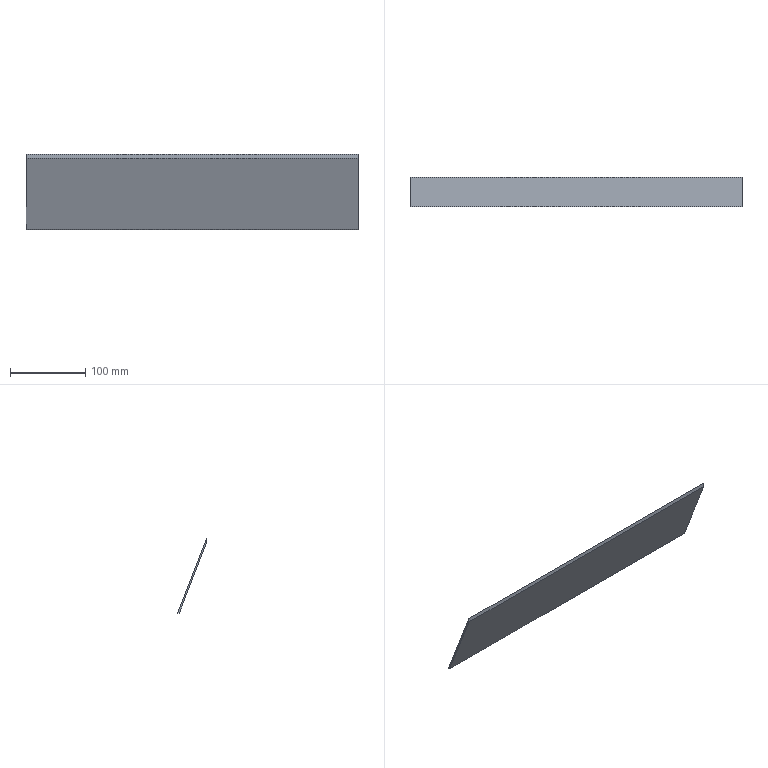Part | NX | features solid 2 | 1 solid | 6 faces | box 440 x 38.653 x 100.695 mm | volume 91707 mm3 | plane 5 | spline 1
STEP:
#1=CARTESIAN_POINT('',(-220.,-25.961,-130.224));
#2=VERTEX_POINT('',#1);
#3=CARTESIAN_POINT('',(-220.,-23.351,-131.441));
#4=VERTEX_POINT('',#3);
#5=CARTESIAN_POINT('',(-220.,730.,-482.734));
#6=DIRECTION('',(0.,-0.9063,0.4226));
#7=VECTOR('',#6,1000.);
#8=LINE('',#5,#7);
#9=EDGE_CURVE('',#2,#4,#8,.F.);
#10=ORIENTED_EDGE('',*,*,#9,.F.);
#11=CARTESIAN_POINT('',(-220.,-62.002,-36.334));
#12=VERTEX_POINT('',#11);
#13=CARTESIAN_POINT('',(-220.,-33.813,-109.769));
#14=DIRECTION('',(0.,-0.3584,0.9336));
#15=VECTOR('',#14,1000.);
#16=LINE('',#13,#15);
#17=EDGE_CURVE('',#2,#12,#16,.T.);
#18=ORIENTED_EDGE('',*,*,#17,.T.);
#19=CARTESIAN_POINT('',(-220.,-62.002,-30.753));
#20=VERTEX_POINT('',#19);
#21=CARTESIAN_POINT('',(-220.,-62.002,-33.544));
#22=DIRECTION('',(0.,0.,1.));
#23=VECTOR('',#22,1000.);
#24=LINE('',#21,#23);
#25=EDGE_CURVE('',#12,#20,#24,.T.);
#26=ORIENTED_EDGE('',*,*,#25,.T.);
#27=CARTESIAN_POINT('',(-220.,-31.946,-109.052));
#28=DIRECTION('',(0.,-0.3584,0.9336));
#29=VECTOR('',#28,1000.);
#30=LINE('',#27,#29);
#31=EDGE_CURVE('',#4,#20,#30,.T.);
#32=ORIENTED_EDGE('',*,*,#31,.F.);
#33=EDGE_LOOP('',(#10,#18,#26,#32));
#34=FACE_BOUND('',#33,.T.);
#35=CARTESIAN_POINT('',(-220.,-33.813,-109.769));
#36=DIRECTION('',(-1.,0.,0.));
#37=DIRECTION('',(0.,-0.3584,0.9336));
#38=AXIS2_PLACEMENT_3D('',#35,#36,#37);
#39=PLANE('',#38);
#40=ADVANCED_FACE('',(#34),#39,.T.);
#41=ORIENTED_EDGE('',*,*,#25,.F.);
#42=CARTESIAN_POINT('',(220.,-62.,-36.338));
#43=VERTEX_POINT('',#42);
#44=CARTESIAN_POINT('',(-220.,-62.002,-36.334));
#45=CARTESIAN_POINT('',(-73.333,-62.009,-36.315));
#46=CARTESIAN_POINT('',(73.333,-62.,-36.338));
#47=CARTESIAN_POINT('',(220.,-62.,-36.338));
#48=B_SPLINE_CURVE_WITH_KNOTS('',3,(#44,#45,#46,#47),.UNSPECIFIED.,.F.,.F.,(4,4),(0.,0.44),.UNSPECIFIED.);
#49=EDGE_CURVE('',#12,#43,#48,.T.);
#50=ORIENTED_EDGE('',*,*,#49,.T.);
#51=CARTESIAN_POINT('',(220.,-62.,-30.758));
#52=VERTEX_POINT('',#51);
#53=CARTESIAN_POINT('',(220.,-62.,-33.548));
#54=DIRECTION('',(0.,0.,1.));
#55=VECTOR('',#54,1000.);
#56=LINE('',#53,#55);
#57=EDGE_CURVE('',#43,#52,#56,.T.);
#58=ORIENTED_EDGE('',*,*,#57,.T.);
#59=CARTESIAN_POINT('',(-220.,-62.002,-30.753));
#60=CARTESIAN_POINT('',(-73.333,-62.009,-30.734));
#61=CARTESIAN_POINT('',(73.333,-62.,-30.758));
#62=CARTESIAN_POINT('',(220.,-62.,-30.758));
#63=B_SPLINE_CURVE_WITH_KNOTS('',3,(#59,#60,#61,#62),.UNSPECIFIED.,.F.,.F.,(4,4),(0.,0.44),.UNSPECIFIED.);
#64=EDGE_CURVE('',#20,#52,#63,.T.);
#65=ORIENTED_EDGE('',*,*,#64,.F.);
#66=EDGE_LOOP('',(#41,#50,#58,#65));
#67=FACE_BOUND('',#66,.T.);
#68=CARTESIAN_POINT('',(-220.,-62.002,-36.372));
#69=CARTESIAN_POINT('',(-220.,-62.002,-30.714));
#70=CARTESIAN_POINT('',(-73.333,-62.009,-36.372));
#71=CARTESIAN_POINT('',(-73.333,-62.009,-30.714));
#72=CARTESIAN_POINT('',(73.333,-62.,-36.372));
#73=CARTESIAN_POINT('',(73.333,-62.,-30.714));
#74=CARTESIAN_POINT('',(220.,-62.,-36.372));
#75=CARTESIAN_POINT('',(220.,-62.,-30.714));
#76=B_SPLINE_SURFACE_WITH_KNOTS('',3,1,((#68,#69),(#70,#71),(#72,#73),(#74,#75)),.SURF_OF_LINEAR_EXTRUSION.,.F.,.F.,.F.,(4,4),(2,2),(0.04348,1.957),(0.,1.),.PIECEWISE_BEZIER_KNOTS.);
#77=ADVANCED_FACE('',(#67),#76,.T.);
#78=ORIENTED_EDGE('',*,*,#57,.F.);
#79=CARTESIAN_POINT('',(220.,-25.961,-130.224));
#80=VERTEX_POINT('',#79);
#81=CARTESIAN_POINT('',(220.,-33.813,-109.769));
#82=DIRECTION('',(0.,-0.3584,0.9336));
#83=VECTOR('',#82,1000.);
#84=LINE('',#81,#83);
#85=EDGE_CURVE('',#80,#43,#84,.T.);
#86=ORIENTED_EDGE('',*,*,#85,.F.);
#87=CARTESIAN_POINT('',(220.,-23.351,-131.441));
#88=VERTEX_POINT('',#87);
#89=CARTESIAN_POINT('',(220.,-40.245,-123.563));
#90=DIRECTION('',(0.,0.9063,-0.4226));
#91=VECTOR('',#90,1000.);
#92=LINE('',#89,#91);
#93=EDGE_CURVE('',#80,#88,#92,.T.);
#94=ORIENTED_EDGE('',*,*,#93,.T.);
#95=CARTESIAN_POINT('',(220.,-31.946,-109.052));
#96=DIRECTION('',(0.,-0.3584,0.9336));
#97=VECTOR('',#96,1000.);
#98=LINE('',#95,#97);
#99=EDGE_CURVE('',#88,#52,#98,.T.);
#100=ORIENTED_EDGE('',*,*,#99,.T.);
#101=EDGE_LOOP('',(#78,#86,#94,#100));
#102=FACE_BOUND('',#101,.T.);
#103=CARTESIAN_POINT('',(220.,-33.813,-109.769));
#104=DIRECTION('',(-1.,0.,0.));
#105=DIRECTION('',(0.,-0.3584,0.9336));
#106=AXIS2_PLACEMENT_3D('',#103,#104,#105);
#107=PLANE('',#106);
#108=ADVANCED_FACE('',(#102),#107,.F.);
#109=ORIENTED_EDGE('',*,*,#99,.F.);
#110=CARTESIAN_POINT('',(300.,-23.351,-131.441));
#111=DIRECTION('',(-1.,0.,0.));
#112=VECTOR('',#111,1000.);
#113=LINE('',#110,#112);
#114=EDGE_CURVE('',#4,#88,#113,.F.);
#115=ORIENTED_EDGE('',*,*,#114,.F.);
#116=ORIENTED_EDGE('',*,*,#31,.T.);
#117=ORIENTED_EDGE('',*,*,#64,.T.);
#118=EDGE_LOOP('',(#109,#115,#116,#117));
#119=FACE_BOUND('',#118,.T.);
#120=CARTESIAN_POINT('',(120.,-31.946,-109.052));
#121=DIRECTION('',(0.,0.9336,0.3584));
#122=DIRECTION('',(0.,-0.3584,0.9336));
#123=AXIS2_PLACEMENT_3D('',#120,#121,#122);
#124=PLANE('',#123);
#125=ADVANCED_FACE('',(#119),#124,.T.);
#126=CARTESIAN_POINT('',(300.,-25.961,-130.224));
#127=DIRECTION('',(-1.,0.,0.));
#128=VECTOR('',#127,1000.);
#129=LINE('',#126,#128);
#130=EDGE_CURVE('',#2,#80,#129,.F.);
#131=ORIENTED_EDGE('',*,*,#130,.F.);
#132=ORIENTED_EDGE('',*,*,#9,.T.);
#133=ORIENTED_EDGE('',*,*,#114,.T.);
#134=ORIENTED_EDGE('',*,*,#93,.F.);
#135=EDGE_LOOP('',(#131,#132,#133,#134));
#136=FACE_BOUND('',#135,.T.);
#137=CARTESIAN_POINT('',(300.,730.,-482.734));
#138=DIRECTION('',(0.,0.4226,0.9063));
#139=DIRECTION('',(0.,-0.9063,0.4226));
#140=AXIS2_PLACEMENT_3D('',#137,#138,#139);
#141=PLANE('',#140);
#142=ADVANCED_FACE('',(#136),#141,.F.);
#143=ORIENTED_EDGE('',*,*,#85,.T.);
#144=ORIENTED_EDGE('',*,*,#49,.F.);
#145=ORIENTED_EDGE('',*,*,#17,.F.);
#146=ORIENTED_EDGE('',*,*,#130,.T.);
#147=EDGE_LOOP('',(#143,#144,#145,#146));
#148=FACE_BOUND('',#147,.T.);
#149=CARTESIAN_POINT('',(120.,-33.813,-109.769));
#150=DIRECTION('',(0.,0.9336,0.3584));
#151=DIRECTION('',(0.,-0.3584,0.9336));
#152=AXIS2_PLACEMENT_3D('',#149,#150,#151);
#153=PLANE('',#152);
#154=ADVANCED_FACE('',(#148),#153,.F.);
#155=CLOSED_SHELL('',(#40,#77,#108,#125,#142,#154));
#156=MANIFOLD_SOLID_BREP('',#155);
#157=(LENGTH_UNIT()NAMED_UNIT(*)SI_UNIT(.MILLI.,.METRE.));
#158=UNCERTAINTY_MEASURE_WITH_UNIT(LENGTH_MEASURE(0.0508),#157,'','');
#159=(NAMED_UNIT(*)PLANE_ANGLE_UNIT()SI_UNIT($,.RADIAN.));
#160=(NAMED_UNIT(*)SI_UNIT($,.STERADIAN.)SOLID_ANGLE_UNIT());
#161=(GEOMETRIC_REPRESENTATION_CONTEXT(3)GLOBAL_UNCERTAINTY_ASSIGNED_CONTEXT((#158))GLOBAL_UNIT_ASSIGNED_CONTEXT((#157,#159,#160))REPRESENTATION_CONTEXT('',''));
#162=ADVANCED_BREP_SHAPE_REPRESENTATION('',(#156),#161);